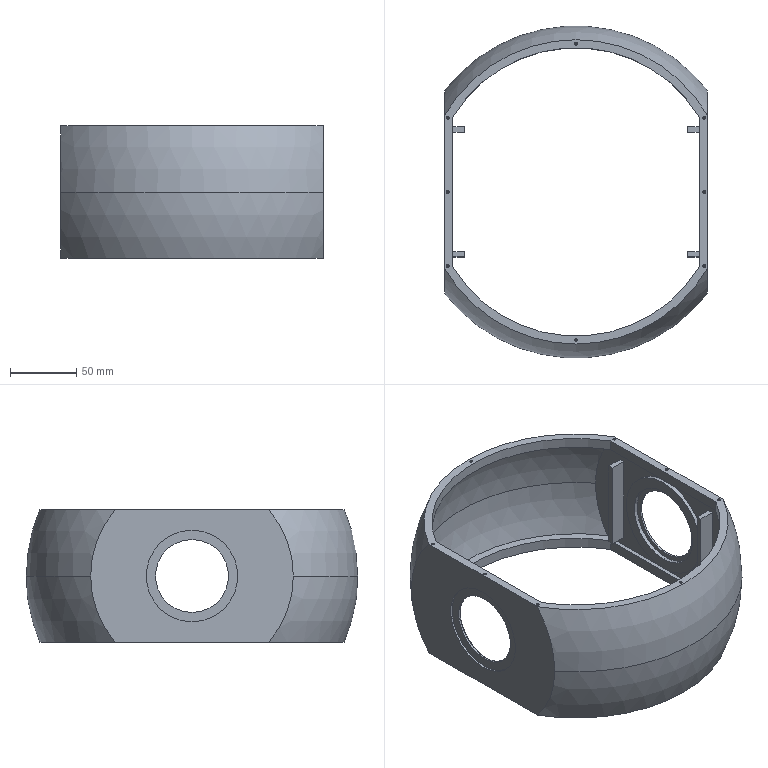Part | SolidWorks | features ICE 7, Cut 4, MirrorPattern 2, CirPattern 1, HoleWzd 1, Revolution 1, Shell 1 | 1 solid | 162 faces | box 198 x 250 x 100 mm | volume 273792 mm3 | cone 64 | cylinder 52 | plane 38 | sphere 8 | commonest cylinder face diameters 1.6 x32 55 x4 61.909 x4 69 x4 78.909 x4 217.129 x4